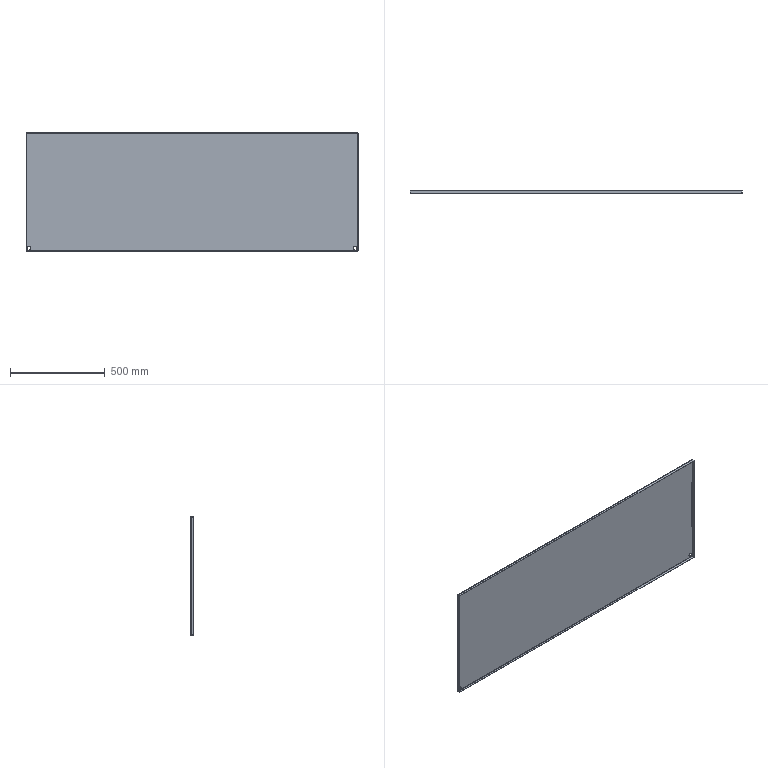Part | SolidWorks | features FlatPattern 1, ICE 1, SMBaseFlange 1, SMMiteredFlange 1, SheetMetal 1 | 1 solid | 42 faces | box 1748 x 15 x 623 mm | volume 1723771 mm3 | plane 22 | cylinder 12 | spline 8 | commonest cylinder face diameters 1.473 x4 4.473 x4 20 x4
STEP:
#1=CARTESIAN_POINT('',(1733.,0.,-598.));
#2=VERTEX_POINT('',#1);
#3=CARTESIAN_POINT('',(1733.,0.,-618.));
#4=VERTEX_POINT('',#3);
#5=CARTESIAN_POINT('',(1733.,0.,-608.));
#6=DIRECTION('',(0.,-1.,0.));
#7=DIRECTION('',(0.,0.,-1.));
#8=AXIS2_PLACEMENT_3D('',#5,#6,#7);
#9=CIRCLE('',#8,10.);
#10=EDGE_CURVE('',#2,#4,#9,.T.);
#11=ORIENTED_EDGE('',*,*,#10,.T.);
#12=CARTESIAN_POINT('',(1733.,1.5,-618.));
#13=VERTEX_POINT('',#12);
#14=CARTESIAN_POINT('',(1733.,-13.5,-618.));
#15=DIRECTION('',(0.,1.,0.));
#16=VECTOR('',#15,1000.);
#17=LINE('',#14,#16);
#18=EDGE_CURVE('',#4,#13,#17,.T.);
#19=ORIENTED_EDGE('',*,*,#18,.T.);
#20=CARTESIAN_POINT('',(1733.,1.5,-598.));
#21=VERTEX_POINT('',#20);
#22=CARTESIAN_POINT('',(1733.,1.5,-608.));
#23=DIRECTION('',(0.,1.,0.));
#24=DIRECTION('',(0.,0.,1.));
#25=AXIS2_PLACEMENT_3D('',#22,#23,#24);
#26=CIRCLE('',#25,10.);
#27=EDGE_CURVE('',#13,#21,#26,.T.);
#28=ORIENTED_EDGE('',*,*,#27,.T.);
#29=CARTESIAN_POINT('',(1733.,-13.5,-598.));
#30=DIRECTION('',(0.,1.,0.));
#31=VECTOR('',#30,1000.);
#32=LINE('',#29,#31);
#33=EDGE_CURVE('',#2,#21,#32,.T.);
#34=ORIENTED_EDGE('',*,*,#33,.F.);
#35=EDGE_LOOP('',(#11,#19,#28,#34));
#36=FACE_OUTER_BOUND('',#35,.T.);
#37=CARTESIAN_POINT('',(1733.,-13.5,-608.));
#38=DIRECTION('',(0.,1.,0.));
#39=DIRECTION('',(0.,0.,1.));
#40=AXIS2_PLACEMENT_3D('',#37,#38,#39);
#41=CYLINDRICAL_SURFACE('',#40,10.);
#42=ADVANCED_FACE('',(#36),#41,.F.);
#43=CARTESIAN_POINT('',(15.,0.,-598.));
#44=VERTEX_POINT('',#43);
#45=CARTESIAN_POINT('',(15.,0.,-618.));
#46=VERTEX_POINT('',#45);
#47=CARTESIAN_POINT('',(15.,0.,-608.));
#48=DIRECTION('',(0.,-1.,0.));
#49=DIRECTION('',(0.,0.,-1.));
#50=AXIS2_PLACEMENT_3D('',#47,#48,#49);
#51=CIRCLE('',#50,10.);
#52=EDGE_CURVE('',#44,#46,#51,.T.);
#53=ORIENTED_EDGE('',*,*,#52,.T.);
#54=CARTESIAN_POINT('',(15.,1.5,-618.));
#55=VERTEX_POINT('',#54);
#56=CARTESIAN_POINT('',(15.,-13.5,-618.));
#57=DIRECTION('',(0.,1.,0.));
#58=VECTOR('',#57,1000.);
#59=LINE('',#56,#58);
#60=EDGE_CURVE('',#46,#55,#59,.T.);
#61=ORIENTED_EDGE('',*,*,#60,.T.);
#62=CARTESIAN_POINT('',(15.,1.5,-598.));
#63=VERTEX_POINT('',#62);
#64=CARTESIAN_POINT('',(15.,1.5,-608.));
#65=DIRECTION('',(0.,1.,0.));
#66=DIRECTION('',(0.,0.,1.));
#67=AXIS2_PLACEMENT_3D('',#64,#65,#66);
#68=CIRCLE('',#67,10.);
#69=EDGE_CURVE('',#55,#63,#68,.T.);
#70=ORIENTED_EDGE('',*,*,#69,.T.);
#71=CARTESIAN_POINT('',(15.,-13.5,-598.));
#72=DIRECTION('',(0.,1.,0.));
#73=VECTOR('',#72,1000.);
#74=LINE('',#71,#73);
#75=EDGE_CURVE('',#44,#63,#74,.T.);
#76=ORIENTED_EDGE('',*,*,#75,.F.);
#77=EDGE_LOOP('',(#53,#61,#70,#76));
#78=FACE_OUTER_BOUND('',#77,.T.);
#79=CARTESIAN_POINT('',(15.,-13.5,-608.));
#80=DIRECTION('',(0.,1.,0.));
#81=DIRECTION('',(0.,0.,1.));
#82=AXIS2_PLACEMENT_3D('',#79,#80,#81);
#83=CYLINDRICAL_SURFACE('',#82,10.);
#84=ADVANCED_FACE('',(#78),#83,.F.);
#85=ORIENTED_EDGE('',*,*,#10,.F.);
#86=CARTESIAN_POINT('',(1733.,0.,-608.));
#87=DIRECTION('',(0.,-1.,0.));
#88=DIRECTION('',(0.,0.,-1.));
#89=AXIS2_PLACEMENT_3D('',#86,#87,#88);
#90=CIRCLE('',#89,10.);
#91=EDGE_CURVE('',#4,#2,#90,.T.);
#92=ORIENTED_EDGE('',*,*,#91,.F.);
#93=EDGE_LOOP('',(#85,#92));
#94=FACE_BOUND('',#93,.T.);
#95=ORIENTED_EDGE('',*,*,#52,.F.);
#96=CARTESIAN_POINT('',(15.,0.,-608.));
#97=DIRECTION('',(0.,-1.,0.));
#98=DIRECTION('',(0.,0.,-1.));
#99=AXIS2_PLACEMENT_3D('',#96,#97,#98);
#100=CIRCLE('',#99,10.);
#101=EDGE_CURVE('',#46,#44,#100,.T.);
#102=ORIENTED_EDGE('',*,*,#101,.F.);
#103=EDGE_LOOP('',(#95,#102));
#104=FACE_BOUND('',#103,.T.);
#105=CARTESIAN_POINT('',(2.237,0.,-620.763));
#106=VERTEX_POINT('',#105);
#107=CARTESIAN_POINT('',(2.237,0.,-2.237));
#108=VERTEX_POINT('',#107);
#109=CARTESIAN_POINT('',(2.237,0.,-623.));
#110=DIRECTION('',(0.,0.,1.));
#111=VECTOR('',#110,1000.);
#112=LINE('',#109,#111);
#113=EDGE_CURVE('',#106,#108,#112,.T.);
#114=ORIENTED_EDGE('',*,*,#113,.F.);
#115=CARTESIAN_POINT('',(1745.763,0.,-620.763));
#116=VERTEX_POINT('',#115);
#117=CARTESIAN_POINT('',(1748.,0.,-620.763));
#118=DIRECTION('',(-1.,0.,0.));
#119=VECTOR('',#118,1000.);
#120=LINE('',#117,#119);
#121=EDGE_CURVE('',#116,#106,#120,.T.);
#122=ORIENTED_EDGE('',*,*,#121,.F.);
#123=CARTESIAN_POINT('',(1745.763,0.,-2.237));
#124=VERTEX_POINT('',#123);
#125=CARTESIAN_POINT('',(1745.763,0.,0.));
#126=DIRECTION('',(0.,0.,-1.));
#127=VECTOR('',#126,1000.);
#128=LINE('',#125,#127);
#129=EDGE_CURVE('',#124,#116,#128,.T.);
#130=ORIENTED_EDGE('',*,*,#129,.F.);
#131=CARTESIAN_POINT('',(-8740.,0.,-2.237));
#132=DIRECTION('',(1.,0.,0.));
#133=VECTOR('',#132,1000.);
#134=LINE('',#131,#133);
#135=EDGE_CURVE('',#108,#124,#134,.T.);
#136=ORIENTED_EDGE('',*,*,#135,.F.);
#137=EDGE_LOOP('',(#114,#122,#130,#136));
#138=FACE_OUTER_BOUND('',#137,.T.);
#139=CARTESIAN_POINT('',(0.,0.,-623.));
#140=DIRECTION('',(0.,-1.,0.));
#141=DIRECTION('',(0.,0.,-1.));
#142=AXIS2_PLACEMENT_3D('',#139,#140,#141);
#143=PLANE('',#142);
#144=ADVANCED_FACE('',(#94,#104,#138),#143,.T.);
#145=CARTESIAN_POINT('',(1733.,1.5,-608.));
#146=DIRECTION('',(0.,1.,0.));
#147=DIRECTION('',(0.,0.,1.));
#148=AXIS2_PLACEMENT_3D('',#145,#146,#147);
#149=CIRCLE('',#148,10.);
#150=EDGE_CURVE('',#21,#13,#149,.T.);
#151=ORIENTED_EDGE('',*,*,#150,.F.);
#152=ORIENTED_EDGE('',*,*,#27,.F.);
#153=EDGE_LOOP('',(#151,#152));
#154=FACE_BOUND('',#153,.T.);
#155=CARTESIAN_POINT('',(15.,1.5,-608.));
#156=DIRECTION('',(0.,1.,0.));
#157=DIRECTION('',(0.,0.,1.));
#158=AXIS2_PLACEMENT_3D('',#155,#156,#157);
#159=CIRCLE('',#158,10.);
#160=EDGE_CURVE('',#63,#55,#159,.T.);
#161=ORIENTED_EDGE('',*,*,#160,.F.);
#162=ORIENTED_EDGE('',*,*,#69,.F.);
#163=EDGE_LOOP('',(#161,#162));
#164=FACE_BOUND('',#163,.T.);
#165=CARTESIAN_POINT('',(1745.763,1.5,-620.763));
#166=VERTEX_POINT('',#165);
#167=CARTESIAN_POINT('',(2.237,1.5,-620.763));
#168=VERTEX_POINT('',#167);
#169=CARTESIAN_POINT('',(1748.,1.5,-620.763));
#170=DIRECTION('',(-1.,0.,0.));
#171=VECTOR('',#170,1000.);
#172=LINE('',#169,#171);
#173=EDGE_CURVE('',#166,#168,#172,.T.);
#174=ORIENTED_EDGE('',*,*,#173,.T.);
#175=CARTESIAN_POINT('',(2.237,1.5,-2.237));
#176=VERTEX_POINT('',#175);
#177=CARTESIAN_POINT('',(2.237,1.5,-623.));
#178=DIRECTION('',(0.,0.,1.));
#179=VECTOR('',#178,1000.);
#180=LINE('',#177,#179);
#181=EDGE_CURVE('',#168,#176,#180,.T.);
#182=ORIENTED_EDGE('',*,*,#181,.T.);
#183=CARTESIAN_POINT('',(1745.763,1.5,-2.237));
#184=VERTEX_POINT('',#183);
#185=CARTESIAN_POINT('',(-8740.,1.5,-2.237));
#186=DIRECTION('',(1.,0.,0.));
#187=VECTOR('',#186,1000.);
#188=LINE('',#185,#187);
#189=EDGE_CURVE('',#176,#184,#188,.T.);
#190=ORIENTED_EDGE('',*,*,#189,.T.);
#191=CARTESIAN_POINT('',(1745.763,1.5,0.));
#192=DIRECTION('',(0.,0.,-1.));
#193=VECTOR('',#192,1000.);
#194=LINE('',#191,#193);
#195=EDGE_CURVE('',#184,#166,#194,.T.);
#196=ORIENTED_EDGE('',*,*,#195,.T.);
#197=EDGE_LOOP('',(#174,#182,#190,#196));
#198=FACE_OUTER_BOUND('',#197,.T.);
#199=CARTESIAN_POINT('',(0.,1.5,-623.));
#200=DIRECTION('',(0.,-1.,0.));
#201=DIRECTION('',(0.,0.,-1.));
#202=AXIS2_PLACEMENT_3D('',#199,#200,#201);
#203=PLANE('',#202);
#204=ADVANCED_FACE('',(#154,#164,#198),#203,.F.);
#205=CARTESIAN_POINT('',(1746.323,-13.5,0.));
#206=VERTEX_POINT('',#205);
#207=CARTESIAN_POINT('',(1746.323,-13.5,-1.5));
#208=VERTEX_POINT('',#207);
#209=CARTESIAN_POINT('',(1746.323,-13.5,0.));
#210=DIRECTION('',(0.,0.,-1.));
#211=VECTOR('',#210,1000.);
#212=LINE('',#209,#211);
#213=EDGE_CURVE('',#206,#208,#212,.T.);
#214=ORIENTED_EDGE('',*,*,#213,.F.);
#215=CARTESIAN_POINT('',(1.677,-13.5,0.));
#216=VERTEX_POINT('',#215);
#217=CARTESIAN_POINT('',(-8740.,-13.5,0.));
#218=DIRECTION('',(1.,0.,0.));
#219=VECTOR('',#218,1000.);
#220=LINE('',#217,#219);
#221=EDGE_CURVE('',#216,#206,#220,.T.);
#222=ORIENTED_EDGE('',*,*,#221,.F.);
#223=CARTESIAN_POINT('',(1.677,-13.5,-1.5));
#224=VERTEX_POINT('',#223);
#225=CARTESIAN_POINT('',(1.677,-13.5,0.));
#226=DIRECTION('',(0.,0.,-1.));
#227=VECTOR('',#226,1000.);
#228=LINE('',#225,#227);
#229=EDGE_CURVE('',#216,#224,#228,.T.);
#230=ORIENTED_EDGE('',*,*,#229,.T.);
#231=CARTESIAN_POINT('',(-8740.,-13.5,-1.5));
#232=DIRECTION('',(1.,0.,0.));
#233=VECTOR('',#232,1000.);
#234=LINE('',#231,#233);
#235=EDGE_CURVE('',#224,#208,#234,.T.);
#236=ORIENTED_EDGE('',*,*,#235,.T.);
#237=EDGE_LOOP('',(#214,#222,#230,#236));
#238=FACE_OUTER_BOUND('',#237,.T.);
#239=CARTESIAN_POINT('',(-8740.,-13.5,0.));
#240=DIRECTION('',(0.,1.,0.));
#241=DIRECTION('',(1.,0.,0.));
#242=AXIS2_PLACEMENT_3D('',#239,#240,#241);
#243=PLANE('',#242);
#244=ADVANCED_FACE('',(#238),#243,.F.);
#245=ORIENTED_EDGE('',*,*,#229,.F.);
#246=CARTESIAN_POINT('',(1.677,-0.7366,0.));
#247=VERTEX_POINT('',#246);
#248=CARTESIAN_POINT('',(1.677,-13.5,0.));
#249=DIRECTION('',(0.,1.,0.));
#250=VECTOR('',#249,1000.);
#251=LINE('',#248,#250);
#252=EDGE_CURVE('',#216,#247,#251,.T.);
#253=ORIENTED_EDGE('',*,*,#252,.T.);
#254=CARTESIAN_POINT('',(1.677,-0.7366,-1.5));
#255=VERTEX_POINT('',#254);
#256=CARTESIAN_POINT('',(1.677,-0.7366,0.));
#257=DIRECTION('',(0.,0.,-1.));
#258=VECTOR('',#257,1000.);
#259=LINE('',#256,#258);
#260=EDGE_CURVE('',#247,#255,#259,.T.);
#261=ORIENTED_EDGE('',*,*,#260,.T.);
#262=CARTESIAN_POINT('',(1.677,-13.5,-1.5));
#263=DIRECTION('',(0.,1.,0.));
#264=VECTOR('',#263,1000.);
#265=LINE('',#262,#264);
#266=EDGE_CURVE('',#224,#255,#265,.T.);
#267=ORIENTED_EDGE('',*,*,#266,.F.);
#268=EDGE_LOOP('',(#245,#253,#261,#267));
#269=FACE_OUTER_BOUND('',#268,.T.);
#270=CARTESIAN_POINT('',(1.677,-13.5,0.));
#271=DIRECTION('',(-1.,0.,0.));
#272=DIRECTION('',(0.,1.,0.));
#273=AXIS2_PLACEMENT_3D('',#270,#271,#272);
#274=PLANE('',#273);
#275=ADVANCED_FACE('',(#269),#274,.T.);
#276=CARTESIAN_POINT('',(1746.323,-0.7366,0.));
#277=VERTEX_POINT('',#276);
#278=CARTESIAN_POINT('',(1746.323,-13.5,0.));
#279=DIRECTION('',(0.,-1.,0.));
#280=VECTOR('',#279,1000.);
#281=LINE('',#278,#280);
#282=EDGE_CURVE('',#277,#206,#281,.T.);
#283=ORIENTED_EDGE('',*,*,#282,.T.);
#284=ORIENTED_EDGE('',*,*,#213,.T.);
#285=CARTESIAN_POINT('',(1746.323,-0.7366,-1.5));
#286=VERTEX_POINT('',#285);
#287=CARTESIAN_POINT('',(1746.323,-13.5,-1.5));
#288=DIRECTION('',(0.,-1.,0.));
#289=VECTOR('',#288,1000.);
#290=LINE('',#287,#289);
#291=EDGE_CURVE('',#286,#208,#290,.T.);
#292=ORIENTED_EDGE('',*,*,#291,.F.);
#293=CARTESIAN_POINT('',(1746.323,-0.7366,0.));
#294=DIRECTION('',(0.,0.,-1.));
#295=VECTOR('',#294,1000.);
#296=LINE('',#293,#295);
#297=EDGE_CURVE('',#277,#286,#296,.T.);
#298=ORIENTED_EDGE('',*,*,#297,.F.);
#299=EDGE_LOOP('',(#283,#284,#292,#298));
#300=FACE_OUTER_BOUND('',#299,.T.);
#301=CARTESIAN_POINT('',(1746.323,-13.5,0.));
#302=DIRECTION('',(-1.,0.,0.));
#303=DIRECTION('',(0.,1.,0.));
#304=AXIS2_PLACEMENT_3D('',#301,#302,#303);
#305=PLANE('',#304);
#306=ADVANCED_FACE('',(#300),#305,.F.);
#307=CARTESIAN_POINT('',(-8740.,-0.7366,-1.5));
#308=DIRECTION('',(1.,0.,0.));
#309=VECTOR('',#308,1000.);
#310=LINE('',#307,#309);
#311=EDGE_CURVE('',#255,#286,#310,.T.);
#312=ORIENTED_EDGE('',*,*,#311,.T.);
#313=ORIENTED_EDGE('',*,*,#291,.T.);
#314=ORIENTED_EDGE('',*,*,#235,.F.);
#315=ORIENTED_EDGE('',*,*,#266,.T.);
#316=EDGE_LOOP('',(#312,#313,#314,#315));
#317=FACE_OUTER_BOUND('',#316,.T.);
#318=CARTESIAN_POINT('',(-8740.,-13.5,-1.5));
#319=DIRECTION('',(0.,0.,-1.));
#320=DIRECTION('',(0.,1.,0.));
#321=AXIS2_PLACEMENT_3D('',#318,#319,#320);
#322=PLANE('',#321);
#323=ADVANCED_FACE('',(#317),#322,.T.);
#324=CARTESIAN_POINT('',(-8740.,-0.7366,0.));
#325=DIRECTION('',(1.,0.,0.));
#326=VECTOR('',#325,1000.);
#327=LINE('',#324,#326);
#328=EDGE_CURVE('',#247,#277,#327,.T.);
#329=ORIENTED_EDGE('',*,*,#328,.F.);
#330=ORIENTED_EDGE('',*,*,#252,.F.);
#331=ORIENTED_EDGE('',*,*,#221,.T.);
#332=ORIENTED_EDGE('',*,*,#282,.F.);
#333=EDGE_LOOP('',(#329,#330,#331,#332));
#334=FACE_OUTER_BOUND('',#333,.T.);
#335=CARTESIAN_POINT('',(-8740.,-13.5,0.));
#336=DIRECTION('',(0.,0.,-1.));
#337=DIRECTION('',(0.,1.,0.));
#338=AXIS2_PLACEMENT_3D('',#335,#336,#337);
#339=PLANE('',#338);
#340=ADVANCED_FACE('',(#334),#339,.F.);
#341=ORIENTED_EDGE('',*,*,#260,.F.);
#342=CARTESIAN_POINT('',(1.677,-0.7366,0.));
#343=CARTESIAN_POINT('',(1.677,0.5736,0.));
#344=CARTESIAN_POINT('',(1.909,1.5,-0.9264));
#345=CARTESIAN_POINT('',(2.237,1.5,-2.237));
#346=(BOUNDED_CURVE()B_SPLINE_CURVE(3,(#342,#343,#344,#345),.UNSPECIFIED.,.F.,.T.)B_SPLINE_CURVE_WITH_KNOTS((4,4),(3.142,4.712),.UNSPECIFIED.)CURVE()GEOMETRIC_REPRESENTATION_ITEM()RATIONAL_B_SPLINE_CURVE((1.,0.8047,0.8047,1.))REPRESENTATION_ITEM(''));
#347=EDGE_CURVE('',#247,#176,#346,.T.);
#348=ORIENTED_EDGE('',*,*,#347,.T.);
#349=CARTESIAN_POINT('',(2.237,1.5,-2.237));
#350=DIRECTION('',(0.,-1.,0.));
#351=VECTOR('',#350,1000.);
#352=LINE('',#349,#351);
#353=EDGE_CURVE('',#176,#108,#352,.T.);
#354=ORIENTED_EDGE('',*,*,#353,.T.);
#355=CARTESIAN_POINT('',(1.677,-0.7366,-1.5));
#356=CARTESIAN_POINT('',(1.677,-0.3051,-1.5));
#357=CARTESIAN_POINT('',(1.909,0.,-1.805));
#358=CARTESIAN_POINT('',(2.237,0.,-2.237));
#359=(BOUNDED_CURVE()B_SPLINE_CURVE(3,(#355,#356,#357,#358),.UNSPECIFIED.,.F.,.F.)B_SPLINE_CURVE_WITH_KNOTS((4,4),(3.142,4.712),.UNSPECIFIED.)CURVE()GEOMETRIC_REPRESENTATION_ITEM()RATIONAL_B_SPLINE_CURVE((1.,0.8047,0.8047,1.))REPRESENTATION_ITEM(''));
#360=EDGE_CURVE('',#255,#108,#359,.T.);
#361=ORIENTED_EDGE('',*,*,#360,.F.);
#362=EDGE_LOOP('',(#341,#348,#354,#361));
#363=FACE_OUTER_BOUND('',#362,.T.);
#364=CARTESIAN_POINT('',(2.796,-0.7366,-2.973));
#365=CARTESIAN_POINT('',(2.796,-0.7366,-3.473));
#366=CARTESIAN_POINT('',(2.796,-0.7366,-3.973));
#367=CARTESIAN_POINT('',(2.796,-0.7366,-4.473));
#368=CARTESIAN_POINT('',(2.796,-2.21,-2.973));
#369=CARTESIAN_POINT('',(2.796,-3.21,-3.473));
#370=CARTESIAN_POINT('',(2.796,-4.21,-3.973));
#371=CARTESIAN_POINT('',(2.796,-5.21,-4.473));
#372=CARTESIAN_POINT('',(1.677,-2.21,-1.5));
#373=CARTESIAN_POINT('',(1.677,-3.21,-1.));
#374=CARTESIAN_POINT('',(1.677,-4.21,-0.5));
#375=CARTESIAN_POINT('',(1.677,-5.21,0.));
#376=CARTESIAN_POINT('',(1.677,-0.7366,-1.5));
#377=CARTESIAN_POINT('',(1.677,-0.7366,-1.));
#378=CARTESIAN_POINT('',(1.677,-0.7366,-0.5));
#379=CARTESIAN_POINT('',(1.677,-0.7366,0.));
#380=CARTESIAN_POINT('',(1.677,0.7366,-1.5));
#381=CARTESIAN_POINT('',(1.677,1.737,-1.));
#382=CARTESIAN_POINT('',(1.677,2.737,-0.5));
#383=CARTESIAN_POINT('',(1.677,3.737,0.));
#384=CARTESIAN_POINT('',(2.796,0.7366,-2.973));
#385=CARTESIAN_POINT('',(2.796,1.737,-3.473));
#386=CARTESIAN_POINT('',(2.796,2.737,-3.973));
#387=CARTESIAN_POINT('',(2.796,3.737,-4.473));
#388=CARTESIAN_POINT('',(2.796,-0.7366,-2.973));
#389=CARTESIAN_POINT('',(2.796,-0.7366,-3.473));
#390=CARTESIAN_POINT('',(2.796,-0.7366,-3.973));
#391=CARTESIAN_POINT('',(2.796,-0.7366,-4.473));
#392=(BOUNDED_SURFACE()B_SPLINE_SURFACE(3,3,((#364,#365,#366,#367),(#368,#369,#370,#371),(#372,#373,#374,#375),(#376,#377,#378,#379),(#380,#381,#382,#383),(#384,#385,#386,#387),(#388,#389,#390,#391)),.UNSPECIFIED.,.T.,.F.,.F.)B_SPLINE_SURFACE_WITH_KNOTS((4,3,4),(4,4),(0.,0.5,1.),(0.,1.),.UNSPECIFIED.)GEOMETRIC_REPRESENTATION_ITEM()RATIONAL_B_SPLINE_SURFACE(((1.,1.,1.,1.),(0.3333,0.3333,0.3333,0.3333),(0.3333,0.3333,0.3333,0.3333),(1.,1.,1.,1.),(0.3333,0.3333,0.3333,0.3333),(0.3333,0.3333,0.3333,0.3333),(1.,1.,1.,1.)))REPRESENTATION_ITEM('')SURFACE());
#393=ADVANCED_FACE('',(#363),#392,.F.);
#394=CARTESIAN_POINT('',(1745.763,1.5,-2.237));
#395=CARTESIAN_POINT('',(1746.091,1.5,-0.9264));
#396=CARTESIAN_POINT('',(1746.323,0.5736,0.));
#397=CARTESIAN_POINT('',(1746.323,-0.7366,0.));
#398=(BOUNDED_CURVE()B_SPLINE_CURVE(3,(#394,#395,#396,#397),.UNSPECIFIED.,.F.,.F.)B_SPLINE_CURVE_WITH_KNOTS((4,4),(4.712,6.283),.UNSPECIFIED.)CURVE()GEOMETRIC_REPRESENTATION_ITEM()RATIONAL_B_SPLINE_CURVE((1.,0.8047,0.8047,1.))REPRESENTATION_ITEM(''));
#399=EDGE_CURVE('',#184,#277,#398,.T.);
#400=ORIENTED_EDGE('',*,*,#399,.T.);
#401=ORIENTED_EDGE('',*,*,#297,.T.);
#402=CARTESIAN_POINT('',(1745.763,0.,-2.237));
#403=CARTESIAN_POINT('',(1746.091,0.,-1.805));
#404=CARTESIAN_POINT('',(1746.323,-0.3051,-1.5));
#405=CARTESIAN_POINT('',(1746.323,-0.7366,-1.5));
#406=(BOUNDED_CURVE()B_SPLINE_CURVE(3,(#402,#403,#404,#405),.UNSPECIFIED.,.F.,.F.)B_SPLINE_CURVE_WITH_KNOTS((4,4),(4.712,6.283),.UNSPECIFIED.)CURVE()GEOMETRIC_REPRESENTATION_ITEM()RATIONAL_B_SPLINE_CURVE((1.,0.8047,0.8047,1.))REPRESENTATION_ITEM(''));
#407=EDGE_CURVE('',#124,#286,#406,.T.);
#408=ORIENTED_EDGE('',*,*,#407,.F.);
#409=CARTESIAN_POINT('',(1745.763,1.5,-2.237));
#410=DIRECTION('',(0.,-1.,0.));
#411=VECTOR('',#410,1000.);
#412=LINE('',#409,#411);
#413=EDGE_CURVE('',#184,#124,#412,.T.);
#414=ORIENTED_EDGE('',*,*,#413,.F.);
#415=EDGE_LOOP('',(#400,#401,#408,#414));
#416=FACE_OUTER_BOUND('',#415,.T.);
#417=CARTESIAN_POINT('',(1746.323,-0.7366,-1.5));
#418=CARTESIAN_POINT('',(1746.323,-0.7366,-1.));
#419=CARTESIAN_POINT('',(1746.323,-0.7366,-0.5));
#420=CARTESIAN_POINT('',(1746.323,-0.7366,0.));
#421=CARTESIAN_POINT('',(1746.323,-2.21,-1.5));
#422=CARTESIAN_POINT('',(1746.323,-3.21,-1.));
#423=CARTESIAN_POINT('',(1746.323,-4.21,-0.5));
#424=CARTESIAN_POINT('',(1746.323,-5.21,0.));
#425=CARTESIAN_POINT('',(1745.204,-2.21,-2.973));
#426=CARTESIAN_POINT('',(1745.204,-3.21,-3.473));
#427=CARTESIAN_POINT('',(1745.204,-4.21,-3.973));
#428=CARTESIAN_POINT('',(1745.204,-5.21,-4.473));
#429=CARTESIAN_POINT('',(1745.204,-0.7366,-2.973));
#430=CARTESIAN_POINT('',(1745.204,-0.7366,-3.473));
#431=CARTESIAN_POINT('',(1745.204,-0.7366,-3.973));
#432=CARTESIAN_POINT('',(1745.204,-0.7366,-4.473));
#433=CARTESIAN_POINT('',(1745.204,0.7366,-2.973));
#434=CARTESIAN_POINT('',(1745.204,1.737,-3.473));
#435=CARTESIAN_POINT('',(1745.204,2.737,-3.973));
#436=CARTESIAN_POINT('',(1745.204,3.737,-4.473));
#437=CARTESIAN_POINT('',(1746.323,0.7366,-1.5));
#438=CARTESIAN_POINT('',(1746.323,1.737,-1.));
#439=CARTESIAN_POINT('',(1746.323,2.737,-0.5));
#440=CARTESIAN_POINT('',(1746.323,3.737,0.));
#441=CARTESIAN_POINT('',(1746.323,-0.7366,-1.5));
#442=CARTESIAN_POINT('',(1746.323,-0.7366,-1.));
#443=CARTESIAN_POINT('',(1746.323,-0.7366,-0.5));
#444=CARTESIAN_POINT('',(1746.323,-0.7366,0.));
#445=(BOUNDED_SURFACE()B_SPLINE_SURFACE(3,3,((#417,#418,#419,#420),(#421,#422,#423,#424),(#425,#426,#427,#428),(#429,#430,#431,#432),(#433,#434,#435,#436),(#437,#438,#439,#440),(#441,#442,#443,#444)),.UNSPECIFIED.,.T.,.F.,.F.)B_SPLINE_SURFACE_WITH_KNOTS((4,3,4),(4,4),(0.,0.5,1.),(0.,1.),.UNSPECIFIED.)GEOMETRIC_REPRESENTATION_ITEM()RATIONAL_B_SPLINE_SURFACE(((1.,1.,1.,1.),(0.3333,0.3333,0.3333,0.3333),(0.3333,0.3333,0.3333,0.3333),(1.,1.,1.,1.),(0.3333,0.3333,0.3333,0.3333),(0.3333,0.3333,0.3333,0.3333),(1.,1.,1.,1.)))REPRESENTATION_ITEM('')SURFACE());
#446=ADVANCED_FACE('',(#416),#445,.F.);
#447=ORIENTED_EDGE('',*,*,#135,.T.);
#448=ORIENTED_EDGE('',*,*,#407,.T.);
#449=ORIENTED_EDGE('',*,*,#311,.F.);
#450=ORIENTED_EDGE('',*,*,#360,.T.);
#451=EDGE_LOOP('',(#447,#448,#449,#450));
#452=FACE_OUTER_BOUND('',#451,.T.);
#453=CARTESIAN_POINT('',(-8740.,-0.7366,-2.237));
#454=DIRECTION('',(1.,0.,0.));
#455=DIRECTION('',(0.,0.,-1.));
#456=AXIS2_PLACEMENT_3D('',#453,#454,#455);
#457=CYLINDRICAL_SURFACE('',#456,0.7366);
#458=ADVANCED_FACE('',(#452),#457,.F.);
#459=ORIENTED_EDGE('',*,*,#189,.F.);
#460=ORIENTED_EDGE('',*,*,#347,.F.);
#461=ORIENTED_EDGE('',*,*,#328,.T.);
#462=ORIENTED_EDGE('',*,*,#399,.F.);
#463=EDGE_LOOP('',(#459,#460,#461,#462));
#464=FACE_OUTER_BOUND('',#463,.T.);
#465=CARTESIAN_POINT('',(-8740.,-0.7366,-2.237));
#466=DIRECTION('',(1.,0.,0.));
#467=DIRECTION('',(0.,0.,-1.));
#468=AXIS2_PLACEMENT_3D('',#465,#466,#467);
#469=CYLINDRICAL_SURFACE('',#468,2.237);
#470=ADVANCED_FACE('',(#464),#469,.T.);
#471=CARTESIAN_POINT('',(1748.,-13.5,-621.323));
#472=VERTEX_POINT('',#471);
#473=CARTESIAN_POINT('',(1746.5,-13.5,-621.323));
#474=VERTEX_POINT('',#473);
#475=CARTESIAN_POINT('',(1748.,-13.5,-621.323));
#476=DIRECTION('',(-1.,0.,0.));
#477=VECTOR('',#476,1000.);
#478=LINE('',#475,#477);
#479=EDGE_CURVE('',#472,#474,#478,.T.);
#480=ORIENTED_EDGE('',*,*,#479,.F.);
#481=CARTESIAN_POINT('',(1748.,-13.5,-1.677));
#482=VERTEX_POINT('',#481);
#483=CARTESIAN_POINT('',(1748.,-13.5,8740.));
#484=DIRECTION('',(0.,0.,-1.));
#485=VECTOR('',#484,1000.);
#486=LINE('',#483,#485);
#487=EDGE_CURVE('',#482,#472,#486,.T.);
#488=ORIENTED_EDGE('',*,*,#487,.F.);
#489=CARTESIAN_POINT('',(1746.5,-13.5,-1.677));
#490=VERTEX_POINT('',#489);
#491=CARTESIAN_POINT('',(1748.,-13.5,-1.677));
#492=DIRECTION('',(-1.,0.,0.));
#493=VECTOR('',#492,1000.);
#494=LINE('',#491,#493);
#495=EDGE_CURVE('',#482,#490,#494,.T.);
#496=ORIENTED_EDGE('',*,*,#495,.T.);
#497=CARTESIAN_POINT('',(1746.5,-13.5,8740.));
#498=DIRECTION('',(0.,0.,-1.));
#499=VECTOR('',#498,1000.);
#500=LINE('',#497,#499);
#501=EDGE_CURVE('',#490,#474,#500,.T.);
#502=ORIENTED_EDGE('',*,*,#501,.T.);
#503=EDGE_LOOP('',(#480,#488,#496,#502));
#504=FACE_OUTER_BOUND('',#503,.T.);
#505=CARTESIAN_POINT('',(1748.,-13.5,8740.));
#506=DIRECTION('',(0.,1.,0.));
#507=DIRECTION('',(0.,0.,-1.));
#508=AXIS2_PLACEMENT_3D('',#505,#506,#507);
#509=PLANE('',#508);
#510=ADVANCED_FACE('',(#504),#509,.F.);
#511=ORIENTED_EDGE('',*,*,#495,.F.);
#512=CARTESIAN_POINT('',(1748.,-0.7366,-1.677));
#513=VERTEX_POINT('',#512);
#514=CARTESIAN_POINT('',(1748.,-13.5,-1.677));
#515=DIRECTION('',(0.,1.,0.));
#516=VECTOR('',#515,1000.);
#517=LINE('',#514,#516);
#518=EDGE_CURVE('',#482,#513,#517,.T.);
#519=ORIENTED_EDGE('',*,*,#518,.T.);
#520=CARTESIAN_POINT('',(1746.5,-0.7366,-1.677));
#521=VERTEX_POINT('',#520);
#522=CARTESIAN_POINT('',(1748.,-0.7366,-1.677));
#523=DIRECTION('',(-1.,0.,0.));
#524=VECTOR('',#523,1000.);
#525=LINE('',#522,#524);
#526=EDGE_CURVE('',#513,#521,#525,.T.);
#527=ORIENTED_EDGE('',*,*,#526,.T.);
#528=CARTESIAN_POINT('',(1746.5,-13.5,-1.677));
#529=DIRECTION('',(0.,1.,0.));
#530=VECTOR('',#529,1000.);
#531=LINE('',#528,#530);
#532=EDGE_CURVE('',#490,#521,#531,.T.);
#533=ORIENTED_EDGE('',*,*,#532,.F.);
#534=EDGE_LOOP('',(#511,#519,#527,#533));
#535=FACE_OUTER_BOUND('',#534,.T.);
#536=CARTESIAN_POINT('',(1748.,-13.5,-1.677));
#537=DIRECTION('',(0.,0.,1.));
#538=DIRECTION('',(0.,1.,0.));
#539=AXIS2_PLACEMENT_3D('',#536,#537,#538);
#540=PLANE('',#539);
#541=ADVANCED_FACE('',(#535),#540,.T.);
#542=CARTESIAN_POINT('',(1748.,-0.7366,-621.323));
#543=VERTEX_POINT('',#542);
#544=CARTESIAN_POINT('',(1748.,-13.5,-621.323));
#545=DIRECTION('',(0.,-1.,0.));
#546=VECTOR('',#545,1000.);
#547=LINE('',#544,#546);
#548=EDGE_CURVE('',#543,#472,#547,.T.);
#549=ORIENTED_EDGE('',*,*,#548,.T.);
#550=ORIENTED_EDGE('',*,*,#479,.T.);
#551=CARTESIAN_POINT('',(1746.5,-0.7366,-621.323));
#552=VERTEX_POINT('',#551);
#553=CARTESIAN_POINT('',(1746.5,-13.5,-621.323));
#554=DIRECTION('',(0.,-1.,0.));
#555=VECTOR('',#554,1000.);
#556=LINE('',#553,#555);
#557=EDGE_CURVE('',#552,#474,#556,.T.);
#558=ORIENTED_EDGE('',*,*,#557,.F.);
#559=CARTESIAN_POINT('',(1748.,-0.7366,-621.323));
#560=DIRECTION('',(-1.,0.,0.));
#561=VECTOR('',#560,1000.);
#562=LINE('',#559,#561);
#563=EDGE_CURVE('',#543,#552,#562,.T.);
#564=ORIENTED_EDGE('',*,*,#563,.F.);
#565=EDGE_LOOP('',(#549,#550,#558,#564));
#566=FACE_OUTER_BOUND('',#565,.T.);
#567=CARTESIAN_POINT('',(1748.,-13.5,-621.323));
#568=DIRECTION('',(0.,0.,1.));
#569=DIRECTION('',(0.,1.,0.));
#570=AXIS2_PLACEMENT_3D('',#567,#568,#569);
#571=PLANE('',#570);
#572=ADVANCED_FACE('',(#566),#571,.F.);
#573=CARTESIAN_POINT('',(1746.5,-0.7366,8740.));
#574=DIRECTION('',(0.,0.,-1.));
#575=VECTOR('',#574,1000.);
#576=LINE('',#573,#575);
#577=EDGE_CURVE('',#521,#552,#576,.T.);
#578=ORIENTED_EDGE('',*,*,#577,.T.);
#579=ORIENTED_EDGE('',*,*,#557,.T.);
#580=ORIENTED_EDGE('',*,*,#501,.F.);
#581=ORIENTED_EDGE('',*,*,#532,.T.);
#582=EDGE_LOOP('',(#578,#579,#580,#581));
#583=FACE_OUTER_BOUND('',#582,.T.);
#584=CARTESIAN_POINT('',(1746.5,-13.5,8740.));
#585=DIRECTION('',(-1.,0.,0.));
#586=DIRECTION('',(0.,1.,0.));
#587=AXIS2_PLACEMENT_3D('',#584,#585,#586);
#588=PLANE('',#587);
#589=ADVANCED_FACE('',(#583),#588,.T.);
#590=CARTESIAN_POINT('',(1748.,-0.7366,8740.));
#591=DIRECTION('',(0.,0.,-1.));
#592=VECTOR('',#591,1000.);
#593=LINE('',#590,#592);
#594=EDGE_CURVE('',#513,#543,#593,.T.);
#595=ORIENTED_EDGE('',*,*,#594,.F.);
#596=ORIENTED_EDGE('',*,*,#518,.F.);
#597=ORIENTED_EDGE('',*,*,#487,.T.);
#598=ORIENTED_EDGE('',*,*,#548,.F.);
#599=EDGE_LOOP('',(#595,#596,#597,#598));
#600=FACE_OUTER_BOUND('',#599,.T.);
#601=CARTESIAN_POINT('',(1748.,-13.5,8740.));
#602=DIRECTION('',(-1.,0.,0.));
#603=DIRECTION('',(0.,1.,0.));
#604=AXIS2_PLACEMENT_3D('',#601,#602,#603);
#605=PLANE('',#604);
#606=ADVANCED_FACE('',(#600),#605,.F.);
#607=ORIENTED_EDGE('',*,*,#526,.F.);
#608=CARTESIAN_POINT('',(1748.,-0.7366,-1.677));
#609=CARTESIAN_POINT('',(1748.,0.5736,-1.677));
#610=CARTESIAN_POINT('',(1747.074,1.5,-1.909));
#611=CARTESIAN_POINT('',(1745.763,1.5,-2.237));
#612=(BOUNDED_CURVE()B_SPLINE_CURVE(3,(#608,#609,#610,#611),.UNSPECIFIED.,.F.,.F.)B_SPLINE_CURVE_WITH_KNOTS((4,4),(3.142,4.712),.UNSPECIFIED.)CURVE()GEOMETRIC_REPRESENTATION_ITEM()RATIONAL_B_SPLINE_CURVE((1.,0.8047,0.8047,1.))REPRESENTATION_ITEM(''));
#613=EDGE_CURVE('',#513,#184,#612,.T.);
#614=ORIENTED_EDGE('',*,*,#613,.T.);
#615=ORIENTED_EDGE('',*,*,#413,.T.);
#616=CARTESIAN_POINT('',(1746.5,-0.7366,-1.677));
#617=CARTESIAN_POINT('',(1746.5,-0.3051,-1.677));
#618=CARTESIAN_POINT('',(1746.195,0.,-1.909));
#619=CARTESIAN_POINT('',(1745.763,0.,-2.237));
#620=(BOUNDED_CURVE()B_SPLINE_CURVE(3,(#616,#617,#618,#619),.UNSPECIFIED.,.F.,.F.)B_SPLINE_CURVE_WITH_KNOTS((4,4),(3.142,4.712),.UNSPECIFIED.)CURVE()GEOMETRIC_REPRESENTATION_ITEM()RATIONAL_B_SPLINE_CURVE((1.,0.8047,0.8047,1.))REPRESENTATION_ITEM(''));
#621=EDGE_CURVE('',#521,#124,#620,.T.);
#622=ORIENTED_EDGE('',*,*,#621,.F.);
#623=EDGE_LOOP('',(#607,#614,#615,#622));
#624=FACE_OUTER_BOUND('',#623,.T.);
#625=CARTESIAN_POINT('',(1745.027,-0.7366,-2.796));
#626=CARTESIAN_POINT('',(1744.527,-0.7366,-2.796));
#627=CARTESIAN_POINT('',(1744.027,-0.7366,-2.796));
#628=CARTESIAN_POINT('',(1743.527,-0.7366,-2.796));
#629=CARTESIAN_POINT('',(1745.027,-2.21,-2.796));
#630=CARTESIAN_POINT('',(1744.527,-3.21,-2.796));
#631=CARTESIAN_POINT('',(1744.027,-4.21,-2.796));
#632=CARTESIAN_POINT('',(1743.527,-5.21,-2.796));
#633=CARTESIAN_POINT('',(1746.5,-2.21,-1.677));
#634=CARTESIAN_POINT('',(1747.,-3.21,-1.677));
#635=CARTESIAN_POINT('',(1747.5,-4.21,-1.677));
#636=CARTESIAN_POINT('',(1748.,-5.21,-1.677));
#637=CARTESIAN_POINT('',(1746.5,-0.7366,-1.677));
#638=CARTESIAN_POINT('',(1747.,-0.7366,-1.677));
#639=CARTESIAN_POINT('',(1747.5,-0.7366,-1.677));
#640=CARTESIAN_POINT('',(1748.,-0.7366,-1.677));
#641=CARTESIAN_POINT('',(1746.5,0.7366,-1.677));
#642=CARTESIAN_POINT('',(1747.,1.737,-1.677));
#643=CARTESIAN_POINT('',(1747.5,2.737,-1.677));
#644=CARTESIAN_POINT('',(1748.,3.737,-1.677));
#645=CARTESIAN_POINT('',(1745.027,0.7366,-2.796));
#646=CARTESIAN_POINT('',(1744.527,1.737,-2.796));
#647=CARTESIAN_POINT('',(1744.027,2.737,-2.796));
#648=CARTESIAN_POINT('',(1743.527,3.737,-2.796));
#649=CARTESIAN_POINT('',(1745.027,-0.7366,-2.796));
#650=CARTESIAN_POINT('',(1744.527,-0.7366,-2.796));
#651=CARTESIAN_POINT('',(1744.027,-0.7366,-2.796));
#652=CARTESIAN_POINT('',(1743.527,-0.7366,-2.796));
#653=(BOUNDED_SURFACE()B_SPLINE_SURFACE(3,3,((#625,#626,#627,#628),(#629,#630,#631,#632),(#633,#634,#635,#636),(#637,#638,#639,#640),(#641,#642,#643,#644),(#645,#646,#647,#648),(#649,#650,#651,#652)),.UNSPECIFIED.,.T.,.F.,.F.)B_SPLINE_SURFACE_WITH_KNOTS((4,3,4),(4,4),(0.,0.5,1.),(0.,1.),.UNSPECIFIED.)GEOMETRIC_REPRESENTATION_ITEM()RATIONAL_B_SPLINE_SURFACE(((1.,1.,1.,1.),(0.3333,0.3333,0.3333,0.3333),(0.3333,0.3333,0.3333,0.3333),(1.,1.,1.,1.),(0.3333,0.3333,0.3333,0.3333),(0.3333,0.3333,0.3333,0.3333),(1.,1.,1.,1.)))REPRESENTATION_ITEM('')SURFACE());
#654=ADVANCED_FACE('',(#624),#653,.F.);
#655=CARTESIAN_POINT('',(1745.763,1.5,-620.763));
#656=CARTESIAN_POINT('',(1747.074,1.5,-621.091));
#657=CARTESIAN_POINT('',(1748.,0.5736,-621.323));
#658=CARTESIAN_POINT('',(1748.,-0.7366,-621.323));
#659=(BOUNDED_CURVE()B_SPLINE_CURVE(3,(#655,#656,#657,#658),.UNSPECIFIED.,.F.,.F.)B_SPLINE_CURVE_WITH_KNOTS((4,4),(4.712,6.283),.UNSPECIFIED.)CURVE()GEOMETRIC_REPRESENTATION_ITEM()RATIONAL_B_SPLINE_CURVE((1.,0.8047,0.8047,1.))REPRESENTATION_ITEM(''));
#660=EDGE_CURVE('',#166,#543,#659,.T.);
#661=ORIENTED_EDGE('',*,*,#660,.T.);
#662=ORIENTED_EDGE('',*,*,#563,.T.);
#663=CARTESIAN_POINT('',(1745.763,0.,-620.763));
#664=CARTESIAN_POINT('',(1746.195,0.,-621.091));
#665=CARTESIAN_POINT('',(1746.5,-0.3051,-621.323));
#666=CARTESIAN_POINT('',(1746.5,-0.7366,-621.323));
#667=(BOUNDED_CURVE()B_SPLINE_CURVE(3,(#663,#664,#665,#666),.UNSPECIFIED.,.F.,.T.)B_SPLINE_CURVE_WITH_KNOTS((4,4),(4.712,6.283),.UNSPECIFIED.)CURVE()GEOMETRIC_REPRESENTATION_ITEM()RATIONAL_B_SPLINE_CURVE((1.,0.8047,0.8047,1.))REPRESENTATION_ITEM(''));
#668=EDGE_CURVE('',#116,#552,#667,.T.);
#669=ORIENTED_EDGE('',*,*,#668,.F.);
#670=CARTESIAN_POINT('',(1745.763,1.5,-620.763));
#671=DIRECTION('',(0.,-1.,0.));
#672=VECTOR('',#671,1000.);
#673=LINE('',#670,#672);
#674=EDGE_CURVE('',#166,#116,#673,.T.);
#675=ORIENTED_EDGE('',*,*,#674,.F.);
#676=EDGE_LOOP('',(#661,#662,#669,#675));
#677=FACE_OUTER_BOUND('',#676,.T.);
#678=CARTESIAN_POINT('',(1746.5,-0.7366,-621.323));
#679=CARTESIAN_POINT('',(1747.,-0.7366,-621.323));
#680=CARTESIAN_POINT('',(1747.5,-0.7366,-621.323));
#681=CARTESIAN_POINT('',(1748.,-0.7366,-621.323));
#682=CARTESIAN_POINT('',(1746.5,-2.21,-621.323));
#683=CARTESIAN_POINT('',(1747.,-3.21,-621.323));
#684=CARTESIAN_POINT('',(1747.5,-4.21,-621.323));
#685=CARTESIAN_POINT('',(1748.,-5.21,-621.323));
#686=CARTESIAN_POINT('',(1745.027,-2.21,-620.204));
#687=CARTESIAN_POINT('',(1744.527,-3.21,-620.204));
#688=CARTESIAN_POINT('',(1744.027,-4.21,-620.204));
#689=CARTESIAN_POINT('',(1743.527,-5.21,-620.204));
#690=CARTESIAN_POINT('',(1745.027,-0.7366,-620.204));
#691=CARTESIAN_POINT('',(1744.527,-0.7366,-620.204));
#692=CARTESIAN_POINT('',(1744.027,-0.7366,-620.204));
#693=CARTESIAN_POINT('',(1743.527,-0.7366,-620.204));
#694=CARTESIAN_POINT('',(1745.027,0.7366,-620.204));
#695=CARTESIAN_POINT('',(1744.527,1.737,-620.204));
#696=CARTESIAN_POINT('',(1744.027,2.737,-620.204));
#697=CARTESIAN_POINT('',(1743.527,3.737,-620.204));
#698=CARTESIAN_POINT('',(1746.5,0.7366,-621.323));
#699=CARTESIAN_POINT('',(1747.,1.737,-621.323));
#700=CARTESIAN_POINT('',(1747.5,2.737,-621.323));
#701=CARTESIAN_POINT('',(1748.,3.737,-621.323));
#702=CARTESIAN_POINT('',(1746.5,-0.7366,-621.323));
#703=CARTESIAN_POINT('',(1747.,-0.7366,-621.323));
#704=CARTESIAN_POINT('',(1747.5,-0.7366,-621.323));
#705=CARTESIAN_POINT('',(1748.,-0.7366,-621.323));
#706=(BOUNDED_SURFACE()B_SPLINE_SURFACE(3,3,((#678,#679,#680,#681),(#682,#683,#684,#685),(#686,#687,#688,#689),(#690,#691,#692,#693),(#694,#695,#696,#697),(#698,#699,#700,#701),(#702,#703,#704,#705)),.UNSPECIFIED.,.T.,.F.,.F.)B_SPLINE_SURFACE_WITH_KNOTS((4,3,4),(4,4),(0.,0.5,1.),(0.,1.),.UNSPECIFIED.)GEOMETRIC_REPRESENTATION_ITEM()RATIONAL_B_SPLINE_SURFACE(((1.,1.,1.,1.),(0.3333,0.3333,0.3333,0.3333),(0.3333,0.3333,0.3333,0.3333),(1.,1.,1.,1.),(0.3333,0.3333,0.3333,0.3333),(0.3333,0.3333,0.3333,0.3333),(1.,1.,1.,1.)))REPRESENTATION_ITEM('')SURFACE());
#707=ADVANCED_FACE('',(#677),#706,.F.);
#708=ORIENTED_EDGE('',*,*,#129,.T.);
#709=ORIENTED_EDGE('',*,*,#668,.T.);
#710=ORIENTED_EDGE('',*,*,#577,.F.);
#711=ORIENTED_EDGE('',*,*,#621,.T.);
#712=EDGE_LOOP('',(#708,#709,#710,#711));
#713=FACE_OUTER_BOUND('',#712,.T.);
#714=CARTESIAN_POINT('',(1745.763,-0.7366,0.));
#715=DIRECTION('',(0.,0.,-1.));
#716=DIRECTION('',(-1.,0.,0.));
#717=AXIS2_PLACEMENT_3D('',#714,#715,#716);
#718=CYLINDRICAL_SURFACE('',#717,0.7366);
#719=ADVANCED_FACE('',(#713),#718,.F.);
#720=ORIENTED_EDGE('',*,*,#195,.F.);
#721=ORIENTED_EDGE('',*,*,#613,.F.);
#722=ORIENTED_EDGE('',*,*,#594,.T.);
#723=ORIENTED_EDGE('',*,*,#660,.F.);
#724=EDGE_LOOP('',(#720,#721,#722,#723));
#725=FACE_OUTER_BOUND('',#724,.T.);
#726=CARTESIAN_POINT('',(1745.763,-0.7366,0.));
#727=DIRECTION('',(0.,0.,-1.));
#728=DIRECTION('',(-1.,0.,0.));
#729=AXIS2_PLACEMENT_3D('',#726,#727,#728);
#730=CYLINDRICAL_SURFACE('',#729,2.237);
#731=ADVANCED_FACE('',(#725),#730,.T.);
#732=CARTESIAN_POINT('',(1.677,-13.5,-623.));
#733=VERTEX_POINT('',#732);
#734=CARTESIAN_POINT('',(1.677,-13.5,-621.5));
#735=VERTEX_POINT('',#734);
#736=CARTESIAN_POINT('',(1.677,-13.5,-623.));
#737=DIRECTION('',(0.,0.,1.));
#738=VECTOR('',#737,1000.);
#739=LINE('',#736,#738);
#740=EDGE_CURVE('',#733,#735,#739,.T.);
#741=ORIENTED_EDGE('',*,*,#740,.F.);
#742=CARTESIAN_POINT('',(1746.323,-13.5,-623.));
#743=VERTEX_POINT('',#742);
#744=CARTESIAN_POINT('',(10488.,-13.5,-623.));
#745=DIRECTION('',(-1.,0.,0.));
#746=VECTOR('',#745,1000.);
#747=LINE('',#744,#746);
#748=EDGE_CURVE('',#743,#733,#747,.T.);
#749=ORIENTED_EDGE('',*,*,#748,.F.);
#750=CARTESIAN_POINT('',(1746.323,-13.5,-621.5));
#751=VERTEX_POINT('',#750);
#752=CARTESIAN_POINT('',(1746.323,-13.5,-623.));
#753=DIRECTION('',(0.,0.,1.));
#754=VECTOR('',#753,1000.);
#755=LINE('',#752,#754);
#756=EDGE_CURVE('',#743,#751,#755,.T.);
#757=ORIENTED_EDGE('',*,*,#756,.T.);
#758=CARTESIAN_POINT('',(10488.,-13.5,-621.5));
#759=DIRECTION('',(-1.,0.,0.));
#760=VECTOR('',#759,1000.);
#761=LINE('',#758,#760);
#762=EDGE_CURVE('',#751,#735,#761,.T.);
#763=ORIENTED_EDGE('',*,*,#762,.T.);
#764=EDGE_LOOP('',(#741,#749,#757,#763));
#765=FACE_OUTER_BOUND('',#764,.T.);
#766=CARTESIAN_POINT('',(10488.,-13.5,-623.));
#767=DIRECTION('',(0.,1.,0.));
#768=DIRECTION('',(-1.,0.,0.));
#769=AXIS2_PLACEMENT_3D('',#766,#767,#768);
#770=PLANE('',#769);
#771=ADVANCED_FACE('',(#765),#770,.F.);
#772=ORIENTED_EDGE('',*,*,#756,.F.);
#773=CARTESIAN_POINT('',(1746.323,-0.7366,-623.));
#774=VERTEX_POINT('',#773);
#775=CARTESIAN_POINT('',(1746.323,-13.5,-623.));
#776=DIRECTION('',(0.,1.,0.));
#777=VECTOR('',#776,1000.);
#778=LINE('',#775,#777);
#779=EDGE_CURVE('',#743,#774,#778,.T.);
#780=ORIENTED_EDGE('',*,*,#779,.T.);
#781=CARTESIAN_POINT('',(1746.323,-0.7366,-621.5));
#782=VERTEX_POINT('',#781);
#783=CARTESIAN_POINT('',(1746.323,-0.7366,-623.));
#784=DIRECTION('',(0.,0.,1.));
#785=VECTOR('',#784,1000.);
#786=LINE('',#783,#785);
#787=EDGE_CURVE('',#774,#782,#786,.T.);
#788=ORIENTED_EDGE('',*,*,#787,.T.);
#789=CARTESIAN_POINT('',(1746.323,-13.5,-621.5));
#790=DIRECTION('',(0.,1.,0.));
#791=VECTOR('',#790,1000.);
#792=LINE('',#789,#791);
#793=EDGE_CURVE('',#751,#782,#792,.T.);
#794=ORIENTED_EDGE('',*,*,#793,.F.);
#795=EDGE_LOOP('',(#772,#780,#788,#794));
#796=FACE_OUTER_BOUND('',#795,.T.);
#797=CARTESIAN_POINT('',(1746.323,-13.5,-623.));
#798=DIRECTION('',(1.,0.,0.));
#799=DIRECTION('',(0.,1.,0.));
#800=AXIS2_PLACEMENT_3D('',#797,#798,#799);
#801=PLANE('',#800);
#802=ADVANCED_FACE('',(#796),#801,.T.);
#803=CARTESIAN_POINT('',(1.677,-0.7366,-623.));
#804=VERTEX_POINT('',#803);
#805=CARTESIAN_POINT('',(1.677,-13.5,-623.));
#806=DIRECTION('',(0.,-1.,0.));
#807=VECTOR('',#806,1000.);
#808=LINE('',#805,#807);
#809=EDGE_CURVE('',#804,#733,#808,.T.);
#810=ORIENTED_EDGE('',*,*,#809,.T.);
#811=ORIENTED_EDGE('',*,*,#740,.T.);
#812=CARTESIAN_POINT('',(1.677,-0.7366,-621.5));
#813=VERTEX_POINT('',#812);
#814=CARTESIAN_POINT('',(1.677,-13.5,-621.5));
#815=DIRECTION('',(0.,-1.,0.));
#816=VECTOR('',#815,1000.);
#817=LINE('',#814,#816);
#818=EDGE_CURVE('',#813,#735,#817,.T.);
#819=ORIENTED_EDGE('',*,*,#818,.F.);
#820=CARTESIAN_POINT('',(1.677,-0.7366,-623.));
#821=DIRECTION('',(0.,0.,1.));
#822=VECTOR('',#821,1000.);
#823=LINE('',#820,#822);
#824=EDGE_CURVE('',#804,#813,#823,.T.);
#825=ORIENTED_EDGE('',*,*,#824,.F.);
#826=EDGE_LOOP('',(#810,#811,#819,#825));
#827=FACE_OUTER_BOUND('',#826,.T.);
#828=CARTESIAN_POINT('',(1.677,-13.5,-623.));
#829=DIRECTION('',(1.,0.,0.));
#830=DIRECTION('',(0.,1.,0.));
#831=AXIS2_PLACEMENT_3D('',#828,#829,#830);
#832=PLANE('',#831);
#833=ADVANCED_FACE('',(#827),#832,.F.);
#834=CARTESIAN_POINT('',(10488.,-0.7366,-621.5));
#835=DIRECTION('',(-1.,0.,0.));
#836=VECTOR('',#835,1000.);
#837=LINE('',#834,#836);
#838=EDGE_CURVE('',#782,#813,#837,.T.);
#839=ORIENTED_EDGE('',*,*,#838,.T.);
#840=ORIENTED_EDGE('',*,*,#818,.T.);
#841=ORIENTED_EDGE('',*,*,#762,.F.);
#842=ORIENTED_EDGE('',*,*,#793,.T.);
#843=EDGE_LOOP('',(#839,#840,#841,#842));
#844=FACE_OUTER_BOUND('',#843,.T.);
#845=CARTESIAN_POINT('',(10488.,-13.5,-621.5));
#846=DIRECTION('',(0.,0.,1.));
#847=DIRECTION('',(0.,1.,0.));
#848=AXIS2_PLACEMENT_3D('',#845,#846,#847);
#849=PLANE('',#848);
#850=ADVANCED_FACE('',(#844),#849,.T.);
#851=CARTESIAN_POINT('',(10488.,-0.7366,-623.));
#852=DIRECTION('',(-1.,0.,0.));
#853=VECTOR('',#852,1000.);
#854=LINE('',#851,#853);
#855=EDGE_CURVE('',#774,#804,#854,.T.);
#856=ORIENTED_EDGE('',*,*,#855,.F.);
#857=ORIENTED_EDGE('',*,*,#779,.F.);
#858=ORIENTED_EDGE('',*,*,#748,.T.);
#859=ORIENTED_EDGE('',*,*,#809,.F.);
#860=EDGE_LOOP('',(#856,#857,#858,#859));
#861=FACE_OUTER_BOUND('',#860,.T.);
#862=CARTESIAN_POINT('',(10488.,-13.5,-623.));
#863=DIRECTION('',(0.,0.,1.));
#864=DIRECTION('',(0.,1.,0.));
#865=AXIS2_PLACEMENT_3D('',#862,#863,#864);
#866=PLANE('',#865);
#867=ADVANCED_FACE('',(#861),#866,.F.);
#868=ORIENTED_EDGE('',*,*,#787,.F.);
#869=CARTESIAN_POINT('',(1746.323,-0.7366,-623.));
#870=CARTESIAN_POINT('',(1746.323,0.5736,-623.));
#871=CARTESIAN_POINT('',(1746.091,1.5,-622.074));
#872=CARTESIAN_POINT('',(1745.763,1.5,-620.763));
#873=(BOUNDED_CURVE()B_SPLINE_CURVE(3,(#869,#870,#871,#872),.UNSPECIFIED.,.F.,.F.)B_SPLINE_CURVE_WITH_KNOTS((4,4),(3.142,4.712),.UNSPECIFIED.)CURVE()GEOMETRIC_REPRESENTATION_ITEM()RATIONAL_B_SPLINE_CURVE((1.,0.8047,0.8047,1.))REPRESENTATION_ITEM(''));
#874=EDGE_CURVE('',#774,#166,#873,.T.);
#875=ORIENTED_EDGE('',*,*,#874,.T.);
#876=ORIENTED_EDGE('',*,*,#674,.T.);
#877=CARTESIAN_POINT('',(1746.323,-0.7366,-621.5));
#878=CARTESIAN_POINT('',(1746.323,-0.3051,-621.5));
#879=CARTESIAN_POINT('',(1746.091,0.,-621.195));
#880=CARTESIAN_POINT('',(1745.763,0.,-620.763));
#881=(BOUNDED_CURVE()B_SPLINE_CURVE(3,(#877,#878,#879,#880),.UNSPECIFIED.,.F.,.F.)B_SPLINE_CURVE_WITH_KNOTS((4,4),(3.142,4.712),.UNSPECIFIED.)CURVE()GEOMETRIC_REPRESENTATION_ITEM()RATIONAL_B_SPLINE_CURVE((1.,0.8047,0.8047,1.))REPRESENTATION_ITEM(''));
#882=EDGE_CURVE('',#782,#116,#881,.T.);
#883=ORIENTED_EDGE('',*,*,#882,.F.);
#884=EDGE_LOOP('',(#868,#875,#876,#883));
#885=FACE_OUTER_BOUND('',#884,.T.);
#886=CARTESIAN_POINT('',(1745.204,-0.7366,-620.027));
#887=CARTESIAN_POINT('',(1745.204,-0.7366,-619.527));
#888=CARTESIAN_POINT('',(1745.204,-0.7366,-619.027));
#889=CARTESIAN_POINT('',(1745.204,-0.7366,-618.527));
#890=CARTESIAN_POINT('',(1745.204,-2.21,-620.027));
#891=CARTESIAN_POINT('',(1745.204,-3.21,-619.527));
#892=CARTESIAN_POINT('',(1745.204,-4.21,-619.027));
#893=CARTESIAN_POINT('',(1745.204,-5.21,-618.527));
#894=CARTESIAN_POINT('',(1746.323,-2.21,-621.5));
#895=CARTESIAN_POINT('',(1746.323,-3.21,-622.));
#896=CARTESIAN_POINT('',(1746.323,-4.21,-622.5));
#897=CARTESIAN_POINT('',(1746.323,-5.21,-623.));
#898=CARTESIAN_POINT('',(1746.323,-0.7366,-621.5));
#899=CARTESIAN_POINT('',(1746.323,-0.7366,-622.));
#900=CARTESIAN_POINT('',(1746.323,-0.7366,-622.5));
#901=CARTESIAN_POINT('',(1746.323,-0.7366,-623.));
#902=CARTESIAN_POINT('',(1746.323,0.7366,-621.5));
#903=CARTESIAN_POINT('',(1746.323,1.737,-622.));
#904=CARTESIAN_POINT('',(1746.323,2.737,-622.5));
#905=CARTESIAN_POINT('',(1746.323,3.737,-623.));
#906=CARTESIAN_POINT('',(1745.204,0.7366,-620.027));
#907=CARTESIAN_POINT('',(1745.204,1.737,-619.527));
#908=CARTESIAN_POINT('',(1745.204,2.737,-619.027));
#909=CARTESIAN_POINT('',(1745.204,3.737,-618.527));
#910=CARTESIAN_POINT('',(1745.204,-0.7366,-620.027));
#911=CARTESIAN_POINT('',(1745.204,-0.7366,-619.527));
#912=CARTESIAN_POINT('',(1745.204,-0.7366,-619.027));
#913=CARTESIAN_POINT('',(1745.204,-0.7366,-618.527));
#914=(BOUNDED_SURFACE()B_SPLINE_SURFACE(3,3,((#886,#887,#888,#889),(#890,#891,#892,#893),(#894,#895,#896,#897),(#898,#899,#900,#901),(#902,#903,#904,#905),(#906,#907,#908,#909),(#910,#911,#912,#913)),.UNSPECIFIED.,.T.,.F.,.F.)B_SPLINE_SURFACE_WITH_KNOTS((4,3,4),(4,4),(0.,0.5,1.),(0.,1.),.UNSPECIFIED.)GEOMETRIC_REPRESENTATION_ITEM()RATIONAL_B_SPLINE_SURFACE(((1.,1.,1.,1.),(0.3333,0.3333,0.3333,0.3333),(0.3333,0.3333,0.3333,0.3333),(1.,1.,1.,1.),(0.3333,0.3333,0.3333,0.3333),(0.3333,0.3333,0.3333,0.3333),(1.,1.,1.,1.)))REPRESENTATION_ITEM('')SURFACE());
#915=ADVANCED_FACE('',(#885),#914,.F.);
#916=CARTESIAN_POINT('',(2.237,1.5,-620.763));
#917=CARTESIAN_POINT('',(1.909,1.5,-622.074));
#918=CARTESIAN_POINT('',(1.677,0.5736,-623.));
#919=CARTESIAN_POINT('',(1.677,-0.7366,-623.));
#920=(BOUNDED_CURVE()B_SPLINE_CURVE(3,(#916,#917,#918,#919),.UNSPECIFIED.,.F.,.F.)B_SPLINE_CURVE_WITH_KNOTS((4,4),(4.712,6.283),.UNSPECIFIED.)CURVE()GEOMETRIC_REPRESENTATION_ITEM()RATIONAL_B_SPLINE_CURVE((1.,0.8047,0.8047,1.))REPRESENTATION_ITEM(''));
#921=EDGE_CURVE('',#168,#804,#920,.T.);
#922=ORIENTED_EDGE('',*,*,#921,.T.);
#923=ORIENTED_EDGE('',*,*,#824,.T.);
#924=CARTESIAN_POINT('',(2.237,0.,-620.763));
#925=CARTESIAN_POINT('',(1.909,0.,-621.195));
#926=CARTESIAN_POINT('',(1.677,-0.3051,-621.5));
#927=CARTESIAN_POINT('',(1.677,-0.7366,-621.5));
#928=(BOUNDED_CURVE()B_SPLINE_CURVE(3,(#924,#925,#926,#927),.UNSPECIFIED.,.F.,.T.)B_SPLINE_CURVE_WITH_KNOTS((4,4),(4.712,6.283),.UNSPECIFIED.)CURVE()GEOMETRIC_REPRESENTATION_ITEM()RATIONAL_B_SPLINE_CURVE((1.,0.8047,0.8047,1.))REPRESENTATION_ITEM(''));
#929=EDGE_CURVE('',#106,#813,#928,.T.);
#930=ORIENTED_EDGE('',*,*,#929,.F.);
#931=CARTESIAN_POINT('',(2.237,1.5,-620.763));
#932=DIRECTION('',(0.,-1.,0.));
#933=VECTOR('',#932,1000.);
#934=LINE('',#931,#933);
#935=EDGE_CURVE('',#168,#106,#934,.T.);
#936=ORIENTED_EDGE('',*,*,#935,.F.);
#937=EDGE_LOOP('',(#922,#923,#930,#936));
#938=FACE_OUTER_BOUND('',#937,.T.);
#939=CARTESIAN_POINT('',(1.677,-0.7366,-621.5));
#940=CARTESIAN_POINT('',(1.677,-0.7366,-622.));
#941=CARTESIAN_POINT('',(1.677,-0.7366,-622.5));
#942=CARTESIAN_POINT('',(1.677,-0.7366,-623.));
#943=CARTESIAN_POINT('',(1.677,-2.21,-621.5));
#944=CARTESIAN_POINT('',(1.677,-3.21,-622.));
#945=CARTESIAN_POINT('',(1.677,-4.21,-622.5));
#946=CARTESIAN_POINT('',(1.677,-5.21,-623.));
#947=CARTESIAN_POINT('',(2.796,-2.21,-620.027));
#948=CARTESIAN_POINT('',(2.796,-3.21,-619.527));
#949=CARTESIAN_POINT('',(2.796,-4.21,-619.027));
#950=CARTESIAN_POINT('',(2.796,-5.21,-618.527));
#951=CARTESIAN_POINT('',(2.796,-0.7366,-620.027));
#952=CARTESIAN_POINT('',(2.796,-0.7366,-619.527));
#953=CARTESIAN_POINT('',(2.796,-0.7366,-619.027));
#954=CARTESIAN_POINT('',(2.796,-0.7366,-618.527));
#955=CARTESIAN_POINT('',(2.796,0.7366,-620.027));
#956=CARTESIAN_POINT('',(2.796,1.737,-619.527));
#957=CARTESIAN_POINT('',(2.796,2.737,-619.027));
#958=CARTESIAN_POINT('',(2.796,3.737,-618.527));
#959=CARTESIAN_POINT('',(1.677,0.7366,-621.5));
#960=CARTESIAN_POINT('',(1.677,1.737,-622.));
#961=CARTESIAN_POINT('',(1.677,2.737,-622.5));
#962=CARTESIAN_POINT('',(1.677,3.737,-623.));
#963=CARTESIAN_POINT('',(1.677,-0.7366,-621.5));
#964=CARTESIAN_POINT('',(1.677,-0.7366,-622.));
#965=CARTESIAN_POINT('',(1.677,-0.7366,-622.5));
#966=CARTESIAN_POINT('',(1.677,-0.7366,-623.));
#967=(BOUNDED_SURFACE()B_SPLINE_SURFACE(3,3,((#939,#940,#941,#942),(#943,#944,#945,#946),(#947,#948,#949,#950),(#951,#952,#953,#954),(#955,#956,#957,#958),(#959,#960,#961,#962),(#963,#964,#965,#966)),.UNSPECIFIED.,.T.,.F.,.F.)B_SPLINE_SURFACE_WITH_KNOTS((4,3,4),(4,4),(0.,0.5,1.),(0.,1.),.UNSPECIFIED.)GEOMETRIC_REPRESENTATION_ITEM()RATIONAL_B_SPLINE_SURFACE(((1.,1.,1.,1.),(0.3333,0.3333,0.3333,0.3333),(0.3333,0.3333,0.3333,0.3333),(1.,1.,1.,1.),(0.3333,0.3333,0.3333,0.3333),(0.3333,0.3333,0.3333,0.3333),(1.,1.,1.,1.)))REPRESENTATION_ITEM('')SURFACE());
#968=ADVANCED_FACE('',(#938),#967,.F.);
#969=ORIENTED_EDGE('',*,*,#121,.T.);
#970=ORIENTED_EDGE('',*,*,#929,.T.);
#971=ORIENTED_EDGE('',*,*,#838,.F.);
#972=ORIENTED_EDGE('',*,*,#882,.T.);
#973=EDGE_LOOP('',(#969,#970,#971,#972));
#974=FACE_OUTER_BOUND('',#973,.T.);
#975=CARTESIAN_POINT('',(1748.,-0.7366,-620.763));
#976=DIRECTION('',(-1.,0.,0.));
#977=DIRECTION('',(0.,0.,1.));
#978=AXIS2_PLACEMENT_3D('',#975,#976,#977);
#979=CYLINDRICAL_SURFACE('',#978,0.7366);
#980=ADVANCED_FACE('',(#974),#979,.F.);
#981=ORIENTED_EDGE('',*,*,#173,.F.);
#982=ORIENTED_EDGE('',*,*,#874,.F.);
#983=ORIENTED_EDGE('',*,*,#855,.T.);
#984=ORIENTED_EDGE('',*,*,#921,.F.);
#985=EDGE_LOOP('',(#981,#982,#983,#984));
#986=FACE_OUTER_BOUND('',#985,.T.);
#987=CARTESIAN_POINT('',(1748.,-0.7366,-620.763));
#988=DIRECTION('',(-1.,0.,0.));
#989=DIRECTION('',(0.,0.,1.));
#990=AXIS2_PLACEMENT_3D('',#987,#988,#989);
#991=CYLINDRICAL_SURFACE('',#990,2.237);
#992=ADVANCED_FACE('',(#986),#991,.T.);
#993=CARTESIAN_POINT('',(0.,-13.5,-1.677));
#994=VERTEX_POINT('',#993);
#995=CARTESIAN_POINT('',(1.5,-13.5,-1.677));
#996=VERTEX_POINT('',#995);
#997=CARTESIAN_POINT('',(0.,-13.5,-1.677));
#998=DIRECTION('',(1.,0.,0.));
#999=VECTOR('',#998,1000.);
#1000=LINE('',#997,#999);
#1001=EDGE_CURVE('',#994,#996,#1000,.T.);
#1002=ORIENTED_EDGE('',*,*,#1001,.F.);
#1003=CARTESIAN_POINT('',(0.,-13.5,-621.323));
#1004=VERTEX_POINT('',#1003);
#1005=CARTESIAN_POINT('',(0.,-13.5,-9363.));
#1006=DIRECTION('',(0.,0.,1.));
#1007=VECTOR('',#1006,1000.);
#1008=LINE('',#1005,#1007);
#1009=EDGE_CURVE('',#1004,#994,#1008,.T.);
#1010=ORIENTED_EDGE('',*,*,#1009,.F.);
#1011=CARTESIAN_POINT('',(1.5,-13.5,-621.323));
#1012=VERTEX_POINT('',#1011);
#1013=CARTESIAN_POINT('',(0.,-13.5,-621.323));
#1014=DIRECTION('',(1.,0.,0.));
#1015=VECTOR('',#1014,1000.);
#1016=LINE('',#1013,#1015);
#1017=EDGE_CURVE('',#1004,#1012,#1016,.T.);
#1018=ORIENTED_EDGE('',*,*,#1017,.T.);
#1019=CARTESIAN_POINT('',(1.5,-13.5,-9363.));
#1020=DIRECTION('',(0.,0.,1.));
#1021=VECTOR('',#1020,1000.);
#1022=LINE('',#1019,#1021);
#1023=EDGE_CURVE('',#1012,#996,#1022,.T.);
#1024=ORIENTED_EDGE('',*,*,#1023,.T.);
#1025=EDGE_LOOP('',(#1002,#1010,#1018,#1024));
#1026=FACE_OUTER_BOUND('',#1025,.T.);
#1027=CARTESIAN_POINT('',(0.,-13.5,-9363.));
#1028=DIRECTION('',(0.,1.,0.));
#1029=DIRECTION('',(0.,0.,1.));
#1030=AXIS2_PLACEMENT_3D('',#1027,#1028,#1029);
#1031=PLANE('',#1030);
#1032=ADVANCED_FACE('',(#1026),#1031,.F.);
#1033=ORIENTED_EDGE('',*,*,#1017,.F.);
#1034=CARTESIAN_POINT('',(0.,-0.7366,-621.323));
#1035=VERTEX_POINT('',#1034);
#1036=CARTESIAN_POINT('',(0.,-13.5,-621.323));
#1037=DIRECTION('',(0.,1.,0.));
#1038=VECTOR('',#1037,1000.);
#1039=LINE('',#1036,#1038);
#1040=EDGE_CURVE('',#1004,#1035,#1039,.T.);
#1041=ORIENTED_EDGE('',*,*,#1040,.T.);
#1042=CARTESIAN_POINT('',(1.5,-0.7366,-621.323));
#1043=VERTEX_POINT('',#1042);
#1044=CARTESIAN_POINT('',(0.,-0.7366,-621.323));
#1045=DIRECTION('',(1.,0.,0.));
#1046=VECTOR('',#1045,1000.);
#1047=LINE('',#1044,#1046);
#1048=EDGE_CURVE('',#1035,#1043,#1047,.T.);
#1049=ORIENTED_EDGE('',*,*,#1048,.T.);
#1050=CARTESIAN_POINT('',(1.5,-13.5,-621.323));
#1051=DIRECTION('',(0.,1.,0.));
#1052=VECTOR('',#1051,1000.);
#1053=LINE('',#1050,#1052);
#1054=EDGE_CURVE('',#1012,#1043,#1053,.T.);
#1055=ORIENTED_EDGE('',*,*,#1054,.F.);
#1056=EDGE_LOOP('',(#1033,#1041,#1049,#1055));
#1057=FACE_OUTER_BOUND('',#1056,.T.);
#1058=CARTESIAN_POINT('',(0.,-13.5,-621.323));
#1059=DIRECTION('',(0.,0.,-1.));
#1060=DIRECTION('',(0.,1.,0.));
#1061=AXIS2_PLACEMENT_3D('',#1058,#1059,#1060);
#1062=PLANE('',#1061);
#1063=ADVANCED_FACE('',(#1057),#1062,.T.);
#1064=CARTESIAN_POINT('',(0.,-0.7366,-1.677));
#1065=VERTEX_POINT('',#1064);
#1066=CARTESIAN_POINT('',(0.,-13.5,-1.677));
#1067=DIRECTION('',(0.,-1.,0.));
#1068=VECTOR('',#1067,1000.);
#1069=LINE('',#1066,#1068);
#1070=EDGE_CURVE('',#1065,#994,#1069,.T.);
#1071=ORIENTED_EDGE('',*,*,#1070,.T.);
#1072=ORIENTED_EDGE('',*,*,#1001,.T.);
#1073=CARTESIAN_POINT('',(1.5,-0.7366,-1.677));
#1074=VERTEX_POINT('',#1073);
#1075=CARTESIAN_POINT('',(1.5,-13.5,-1.677));
#1076=DIRECTION('',(0.,-1.,0.));
#1077=VECTOR('',#1076,1000.);
#1078=LINE('',#1075,#1077);
#1079=EDGE_CURVE('',#1074,#996,#1078,.T.);
#1080=ORIENTED_EDGE('',*,*,#1079,.F.);
#1081=CARTESIAN_POINT('',(0.,-0.7366,-1.677));
#1082=DIRECTION('',(1.,0.,0.));
#1083=VECTOR('',#1082,1000.);
#1084=LINE('',#1081,#1083);
#1085=EDGE_CURVE('',#1065,#1074,#1084,.T.);
#1086=ORIENTED_EDGE('',*,*,#1085,.F.);
#1087=EDGE_LOOP('',(#1071,#1072,#1080,#1086));
#1088=FACE_OUTER_BOUND('',#1087,.T.);
#1089=CARTESIAN_POINT('',(0.,-13.5,-1.677));
#1090=DIRECTION('',(0.,0.,-1.));
#1091=DIRECTION('',(0.,1.,0.));
#1092=AXIS2_PLACEMENT_3D('',#1089,#1090,#1091);
#1093=PLANE('',#1092);
#1094=ADVANCED_FACE('',(#1088),#1093,.F.);
#1095=CARTESIAN_POINT('',(1.5,-0.7366,-9363.));
#1096=DIRECTION('',(0.,0.,1.));
#1097=VECTOR('',#1096,1000.);
#1098=LINE('',#1095,#1097);
#1099=EDGE_CURVE('',#1043,#1074,#1098,.T.);
#1100=ORIENTED_EDGE('',*,*,#1099,.T.);
#1101=ORIENTED_EDGE('',*,*,#1079,.T.);
#1102=ORIENTED_EDGE('',*,*,#1023,.F.);
#1103=ORIENTED_EDGE('',*,*,#1054,.T.);
#1104=EDGE_LOOP('',(#1100,#1101,#1102,#1103));
#1105=FACE_OUTER_BOUND('',#1104,.T.);
#1106=CARTESIAN_POINT('',(1.5,-13.5,-9363.));
#1107=DIRECTION('',(1.,0.,0.));
#1108=DIRECTION('',(0.,1.,0.));
#1109=AXIS2_PLACEMENT_3D('',#1106,#1107,#1108);
#1110=PLANE('',#1109);
#1111=ADVANCED_FACE('',(#1105),#1110,.T.);
#1112=CARTESIAN_POINT('',(0.,-0.7366,-9363.));
#1113=DIRECTION('',(0.,0.,1.));
#1114=VECTOR('',#1113,1000.);
#1115=LINE('',#1112,#1114);
#1116=EDGE_CURVE('',#1035,#1065,#1115,.T.);
#1117=ORIENTED_EDGE('',*,*,#1116,.F.);
#1118=ORIENTED_EDGE('',*,*,#1040,.F.);
#1119=ORIENTED_EDGE('',*,*,#1009,.T.);
#1120=ORIENTED_EDGE('',*,*,#1070,.F.);
#1121=EDGE_LOOP('',(#1117,#1118,#1119,#1120));
#1122=FACE_OUTER_BOUND('',#1121,.T.);
#1123=CARTESIAN_POINT('',(0.,-13.5,-9363.));
#1124=DIRECTION('',(1.,0.,0.));
#1125=DIRECTION('',(0.,1.,0.));
#1126=AXIS2_PLACEMENT_3D('',#1123,#1124,#1125);
#1127=PLANE('',#1126);
#1128=ADVANCED_FACE('',(#1122),#1127,.F.);
#1129=ORIENTED_EDGE('',*,*,#1048,.F.);
#1130=CARTESIAN_POINT('',(0.,-0.7366,-621.323));
#1131=CARTESIAN_POINT('',(0.,0.5736,-621.323));
#1132=CARTESIAN_POINT('',(0.9264,1.5,-621.091));
#1133=CARTESIAN_POINT('',(2.237,1.5,-620.763));
#1134=(BOUNDED_CURVE()B_SPLINE_CURVE(3,(#1130,#1131,#1132,#1133),.UNSPECIFIED.,.F.,.F.)B_SPLINE_CURVE_WITH_KNOTS((4,4),(3.142,4.712),.UNSPECIFIED.)CURVE()GEOMETRIC_REPRESENTATION_ITEM()RATIONAL_B_SPLINE_CURVE((1.,0.8047,0.8047,1.))REPRESENTATION_ITEM(''));
#1135=EDGE_CURVE('',#1035,#168,#1134,.T.);
#1136=ORIENTED_EDGE('',*,*,#1135,.T.);
#1137=ORIENTED_EDGE('',*,*,#935,.T.);
#1138=CARTESIAN_POINT('',(1.5,-0.7366,-621.323));
#1139=CARTESIAN_POINT('',(1.5,-0.3051,-621.323));
#1140=CARTESIAN_POINT('',(1.805,0.,-621.091));
#1141=CARTESIAN_POINT('',(2.237,0.,-620.763));
#1142=(BOUNDED_CURVE()B_SPLINE_CURVE(3,(#1138,#1139,#1140,#1141),.UNSPECIFIED.,.F.,.F.)B_SPLINE_CURVE_WITH_KNOTS((4,4),(3.142,4.712),.UNSPECIFIED.)CURVE()GEOMETRIC_REPRESENTATION_ITEM()RATIONAL_B_SPLINE_CURVE((1.,0.8047,0.8047,1.))REPRESENTATION_ITEM(''));
#1143=EDGE_CURVE('',#1043,#106,#1142,.T.);
#1144=ORIENTED_EDGE('',*,*,#1143,.F.);
#1145=EDGE_LOOP('',(#1129,#1136,#1137,#1144));
#1146=FACE_OUTER_BOUND('',#1145,.T.);
#1147=CARTESIAN_POINT('',(2.973,-0.7366,-620.204));
#1148=CARTESIAN_POINT('',(3.473,-0.7366,-620.204));
#1149=CARTESIAN_POINT('',(3.973,-0.7366,-620.204));
#1150=CARTESIAN_POINT('',(4.473,-0.7366,-620.204));
#1151=CARTESIAN_POINT('',(2.973,-2.21,-620.204));
#1152=CARTESIAN_POINT('',(3.473,-3.21,-620.204));
#1153=CARTESIAN_POINT('',(3.973,-4.21,-620.204));
#1154=CARTESIAN_POINT('',(4.473,-5.21,-620.204));
#1155=CARTESIAN_POINT('',(1.5,-2.21,-621.323));
#1156=CARTESIAN_POINT('',(1.,-3.21,-621.323));
#1157=CARTESIAN_POINT('',(0.5,-4.21,-621.323));
#1158=CARTESIAN_POINT('',(0.,-5.21,-621.323));
#1159=CARTESIAN_POINT('',(1.5,-0.7366,-621.323));
#1160=CARTESIAN_POINT('',(1.,-0.7366,-621.323));
#1161=CARTESIAN_POINT('',(0.5,-0.7366,-621.323));
#1162=CARTESIAN_POINT('',(0.,-0.7366,-621.323));
#1163=CARTESIAN_POINT('',(1.5,0.7366,-621.323));
#1164=CARTESIAN_POINT('',(1.,1.737,-621.323));
#1165=CARTESIAN_POINT('',(0.5,2.737,-621.323));
#1166=CARTESIAN_POINT('',(0.,3.737,-621.323));
#1167=CARTESIAN_POINT('',(2.973,0.7366,-620.204));
#1168=CARTESIAN_POINT('',(3.473,1.737,-620.204));
#1169=CARTESIAN_POINT('',(3.973,2.737,-620.204));
#1170=CARTESIAN_POINT('',(4.473,3.737,-620.204));
#1171=CARTESIAN_POINT('',(2.973,-0.7366,-620.204));
#1172=CARTESIAN_POINT('',(3.473,-0.7366,-620.204));
#1173=CARTESIAN_POINT('',(3.973,-0.7366,-620.204));
#1174=CARTESIAN_POINT('',(4.473,-0.7366,-620.204));
#1175=(BOUNDED_SURFACE()B_SPLINE_SURFACE(3,3,((#1147,#1148,#1149,#1150),(#1151,#1152,#1153,#1154),(#1155,#1156,#1157,#1158),(#1159,#1160,#1161,#1162),(#1163,#1164,#1165,#1166),(#1167,#1168,#1169,#1170),(#1171,#1172,#1173,#1174)),.UNSPECIFIED.,.T.,.F.,.F.)B_SPLINE_SURFACE_WITH_KNOTS((4,3,4),(4,4),(0.,0.5,1.),(0.,1.),.UNSPECIFIED.)GEOMETRIC_REPRESENTATION_ITEM()RATIONAL_B_SPLINE_SURFACE(((1.,1.,1.,1.),(0.3333,0.3333,0.3333,0.3333),(0.3333,0.3333,0.3333,0.3333),(1.,1.,1.,1.),(0.3333,0.3333,0.3333,0.3333),(0.3333,0.3333,0.3333,0.3333),(1.,1.,1.,1.)))REPRESENTATION_ITEM('')SURFACE());
#1176=ADVANCED_FACE('',(#1146),#1175,.F.);
#1177=CARTESIAN_POINT('',(2.237,1.5,-2.237));
#1178=CARTESIAN_POINT('',(0.9264,1.5,-1.909));
#1179=CARTESIAN_POINT('',(0.,0.5736,-1.677));
#1180=CARTESIAN_POINT('',(0.,-0.7366,-1.677));
#1181=(BOUNDED_CURVE()B_SPLINE_CURVE(3,(#1177,#1178,#1179,#1180),.UNSPECIFIED.,.F.,.F.)B_SPLINE_CURVE_WITH_KNOTS((4,4),(4.712,6.283),.UNSPECIFIED.)CURVE()GEOMETRIC_REPRESENTATION_ITEM()RATIONAL_B_SPLINE_CURVE((1.,0.8047,0.8047,1.))REPRESENTATION_ITEM(''));
#1182=EDGE_CURVE('',#176,#1065,#1181,.T.);
#1183=ORIENTED_EDGE('',*,*,#1182,.T.);
#1184=ORIENTED_EDGE('',*,*,#1085,.T.);
#1185=CARTESIAN_POINT('',(2.237,0.,-2.237));
#1186=CARTESIAN_POINT('',(1.805,0.,-1.909));
#1187=CARTESIAN_POINT('',(1.5,-0.3051,-1.677));
#1188=CARTESIAN_POINT('',(1.5,-0.7366,-1.677));
#1189=(BOUNDED_CURVE()B_SPLINE_CURVE(3,(#1185,#1186,#1187,#1188),.UNSPECIFIED.,.F.,.T.)B_SPLINE_CURVE_WITH_KNOTS((4,4),(4.712,6.283),.UNSPECIFIED.)CURVE()GEOMETRIC_REPRESENTATION_ITEM()RATIONAL_B_SPLINE_CURVE((1.,0.8047,0.8047,1.))REPRESENTATION_ITEM(''));
#1190=EDGE_CURVE('',#108,#1074,#1189,.T.);
#1191=ORIENTED_EDGE('',*,*,#1190,.F.);
#1192=ORIENTED_EDGE('',*,*,#353,.F.);
#1193=EDGE_LOOP('',(#1183,#1184,#1191,#1192));
#1194=FACE_OUTER_BOUND('',#1193,.T.);
#1195=CARTESIAN_POINT('',(1.5,-0.7366,-1.677));
#1196=CARTESIAN_POINT('',(1.,-0.7366,-1.677));
#1197=CARTESIAN_POINT('',(0.5,-0.7366,-1.677));
#1198=CARTESIAN_POINT('',(0.,-0.7366,-1.677));
#1199=CARTESIAN_POINT('',(1.5,-2.21,-1.677));
#1200=CARTESIAN_POINT('',(1.,-3.21,-1.677));
#1201=CARTESIAN_POINT('',(0.5,-4.21,-1.677));
#1202=CARTESIAN_POINT('',(0.,-5.21,-1.677));
#1203=CARTESIAN_POINT('',(2.973,-2.21,-2.796));
#1204=CARTESIAN_POINT('',(3.473,-3.21,-2.796));
#1205=CARTESIAN_POINT('',(3.973,-4.21,-2.796));
#1206=CARTESIAN_POINT('',(4.473,-5.21,-2.796));
#1207=CARTESIAN_POINT('',(2.973,-0.7366,-2.796));
#1208=CARTESIAN_POINT('',(3.473,-0.7366,-2.796));
#1209=CARTESIAN_POINT('',(3.973,-0.7366,-2.796));
#1210=CARTESIAN_POINT('',(4.473,-0.7366,-2.796));
#1211=CARTESIAN_POINT('',(2.973,0.7366,-2.796));
#1212=CARTESIAN_POINT('',(3.473,1.737,-2.796));
#1213=CARTESIAN_POINT('',(3.973,2.737,-2.796));
#1214=CARTESIAN_POINT('',(4.473,3.737,-2.796));
#1215=CARTESIAN_POINT('',(1.5,0.7366,-1.677));
#1216=CARTESIAN_POINT('',(1.,1.737,-1.677));
#1217=CARTESIAN_POINT('',(0.5,2.737,-1.677));
#1218=CARTESIAN_POINT('',(0.,3.737,-1.677));
#1219=CARTESIAN_POINT('',(1.5,-0.7366,-1.677));
#1220=CARTESIAN_POINT('',(1.,-0.7366,-1.677));
#1221=CARTESIAN_POINT('',(0.5,-0.7366,-1.677));
#1222=CARTESIAN_POINT('',(0.,-0.7366,-1.677));
#1223=(BOUNDED_SURFACE()B_SPLINE_SURFACE(3,3,((#1195,#1196,#1197,#1198),(#1199,#1200,#1201,#1202),(#1203,#1204,#1205,#1206),(#1207,#1208,#1209,#1210),(#1211,#1212,#1213,#1214),(#1215,#1216,#1217,#1218),(#1219,#1220,#1221,#1222)),.UNSPECIFIED.,.T.,.F.,.F.)B_SPLINE_SURFACE_WITH_KNOTS((4,3,4),(4,4),(0.,0.5,1.),(0.,1.),.UNSPECIFIED.)GEOMETRIC_REPRESENTATION_ITEM()RATIONAL_B_SPLINE_SURFACE(((1.,1.,1.,1.),(0.3333,0.3333,0.3333,0.3333),(0.3333,0.3333,0.3333,0.3333),(1.,1.,1.,1.),(0.3333,0.3333,0.3333,0.3333),(0.3333,0.3333,0.3333,0.3333),(1.,1.,1.,1.)))REPRESENTATION_ITEM('')SURFACE());
#1224=ADVANCED_FACE('',(#1194),#1223,.F.);
#1225=ORIENTED_EDGE('',*,*,#113,.T.);
#1226=ORIENTED_EDGE('',*,*,#1190,.T.);
#1227=ORIENTED_EDGE('',*,*,#1099,.F.);
#1228=ORIENTED_EDGE('',*,*,#1143,.T.);
#1229=EDGE_LOOP('',(#1225,#1226,#1227,#1228));
#1230=FACE_OUTER_BOUND('',#1229,.T.);
#1231=CARTESIAN_POINT('',(2.237,-0.7366,-623.));
#1232=DIRECTION('',(0.,0.,1.));
#1233=DIRECTION('',(1.,0.,0.));
#1234=AXIS2_PLACEMENT_3D('',#1231,#1232,#1233);
#1235=CYLINDRICAL_SURFACE('',#1234,0.7366);
#1236=ADVANCED_FACE('',(#1230),#1235,.F.);
#1237=ORIENTED_EDGE('',*,*,#181,.F.);
#1238=ORIENTED_EDGE('',*,*,#1135,.F.);
#1239=ORIENTED_EDGE('',*,*,#1116,.T.);
#1240=ORIENTED_EDGE('',*,*,#1182,.F.);
#1241=EDGE_LOOP('',(#1237,#1238,#1239,#1240));
#1242=FACE_OUTER_BOUND('',#1241,.T.);
#1243=CARTESIAN_POINT('',(2.237,-0.7366,-623.));
#1244=DIRECTION('',(0.,0.,1.));
#1245=DIRECTION('',(1.,0.,0.));
#1246=AXIS2_PLACEMENT_3D('',#1243,#1244,#1245);
#1247=CYLINDRICAL_SURFACE('',#1246,2.237);
#1248=ADVANCED_FACE('',(#1242),#1247,.T.);
#1249=ORIENTED_EDGE('',*,*,#60,.F.);
#1250=ORIENTED_EDGE('',*,*,#101,.T.);
#1251=ORIENTED_EDGE('',*,*,#75,.T.);
#1252=ORIENTED_EDGE('',*,*,#160,.T.);
#1253=EDGE_LOOP('',(#1249,#1250,#1251,#1252));
#1254=FACE_OUTER_BOUND('',#1253,.T.);
#1255=CARTESIAN_POINT('',(15.,-13.5,-608.));
#1256=DIRECTION('',(0.,1.,0.));
#1257=DIRECTION('',(0.,0.,1.));
#1258=AXIS2_PLACEMENT_3D('',#1255,#1256,#1257);
#1259=CYLINDRICAL_SURFACE('',#1258,10.);
#1260=ADVANCED_FACE('',(#1254),#1259,.F.);
#1261=ORIENTED_EDGE('',*,*,#18,.F.);
#1262=ORIENTED_EDGE('',*,*,#91,.T.);
#1263=ORIENTED_EDGE('',*,*,#33,.T.);
#1264=ORIENTED_EDGE('',*,*,#150,.T.);
#1265=EDGE_LOOP('',(#1261,#1262,#1263,#1264));
#1266=FACE_OUTER_BOUND('',#1265,.T.);
#1267=CARTESIAN_POINT('',(1733.,-13.5,-608.));
#1268=DIRECTION('',(0.,1.,0.));
#1269=DIRECTION('',(0.,0.,1.));
#1270=AXIS2_PLACEMENT_3D('',#1267,#1268,#1269);
#1271=CYLINDRICAL_SURFACE('',#1270,10.);
#1272=ADVANCED_FACE('',(#1266),#1271,.F.);
#1273=CLOSED_SHELL('',(#42,#84,#144,#204,#244,#275,#306,#323,#340,#393,#446,#458,#470,#510,#541,#572,#589,#606,#654,#707,#719,#731,#771,#802,#833,#850,#867,#915,#968,#980,#992,#1032,#1063,#1094,#1111,#1128,#1176,#1224,#1236,#1248,#1260,#1272));
#1274=MANIFOLD_SOLID_BREP('',#1273);
#1275=CARTESIAN_POINT('',(0.,0.,0.));
#1276=DIRECTION('',(0.,0.,1.));
#1277=DIRECTION('',(1.,0.,0.));
#1278=AXIS2_PLACEMENT_3D('',#1275,#1276,#1277);
#1279=(LENGTH_UNIT()NAMED_UNIT(*)SI_UNIT(.MILLI.,.METRE.));
#1280=UNCERTAINTY_MEASURE_WITH_UNIT(LENGTH_MEASURE(0.00001),#1279,'','');
#1281=(NAMED_UNIT(*)PLANE_ANGLE_UNIT()SI_UNIT($,.RADIAN.));
#1282=(NAMED_UNIT(*)SI_UNIT($,.STERADIAN.)SOLID_ANGLE_UNIT());
#1283=(GEOMETRIC_REPRESENTATION_CONTEXT(3)GLOBAL_UNCERTAINTY_ASSIGNED_CONTEXT((#1280))GLOBAL_UNIT_ASSIGNED_CONTEXT((#1279,#1281,#1282))REPRESENTATION_CONTEXT('',''));
#1284=ADVANCED_BREP_SHAPE_REPRESENTATION('',(#1274,#1278),#1283);